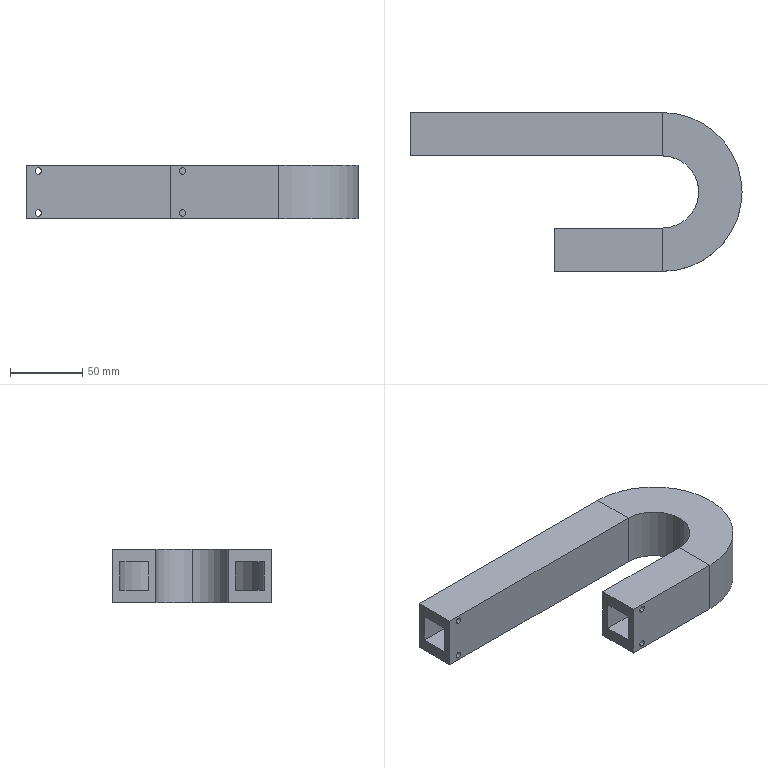Part | SolidWorks | features HoleWzd 2, Sweep 1 | 1 solid | 38 faces | box 230 x 110 x 37 mm | volume 264813 mm3 | plane 22 | cylinder 16 | commonest cylinder face diameters 4.5 x8 50 x2 60 x2 100 x2 110 x2
STEP:
#1=CARTESIAN_POINT('',(-91.5,65.,-12.25));
#2=VERTEX_POINT('',#1);
#3=CARTESIAN_POINT('',(-91.5,65.,-16.75));
#4=VERTEX_POINT('',#3);
#5=CARTESIAN_POINT('',(-91.5,65.,-14.5));
#6=DIRECTION('',(0.,-1.,0.));
#7=DIRECTION('',(1.,0.,0.));
#8=AXIS2_PLACEMENT_3D('',#5,#6,#7);
#9=CIRCLE('',#8,2.25);
#10=EDGE_CURVE('',#2,#4,#9,.T.);
#11=ORIENTED_EDGE('',*,*,#10,.T.);
#12=CARTESIAN_POINT('',(-91.5,95.,-16.75));
#13=VERTEX_POINT('',#12);
#14=CARTESIAN_POINT('',(-91.5,95.,-16.75));
#15=DIRECTION('',(0.,1.,0.));
#16=VECTOR('',#15,1000.);
#17=LINE('',#14,#16);
#18=EDGE_CURVE('',#4,#13,#17,.T.);
#19=ORIENTED_EDGE('',*,*,#18,.T.);
#20=CARTESIAN_POINT('',(-91.5,95.,-12.25));
#21=VERTEX_POINT('',#20);
#22=CARTESIAN_POINT('',(-91.5,95.,-14.5));
#23=DIRECTION('',(0.,1.,0.));
#24=DIRECTION('',(0.,0.,1.));
#25=AXIS2_PLACEMENT_3D('',#22,#23,#24);
#26=CIRCLE('',#25,2.25);
#27=EDGE_CURVE('',#13,#21,#26,.T.);
#28=ORIENTED_EDGE('',*,*,#27,.T.);
#29=CARTESIAN_POINT('',(-91.5,95.,-12.25));
#30=DIRECTION('',(0.,1.,0.));
#31=VECTOR('',#30,1000.);
#32=LINE('',#29,#31);
#33=EDGE_CURVE('',#2,#21,#32,.T.);
#34=ORIENTED_EDGE('',*,*,#33,.F.);
#35=EDGE_LOOP('',(#11,#19,#28,#34));
#36=FACE_OUTER_BOUND('',#35,.T.);
#37=CARTESIAN_POINT('',(-91.5,95.,-14.5));
#38=DIRECTION('',(0.,1.,0.));
#39=DIRECTION('',(0.,0.,1.));
#40=AXIS2_PLACEMENT_3D('',#37,#38,#39);
#41=CYLINDRICAL_SURFACE('',#40,2.25);
#42=ADVANCED_FACE('',(#36),#41,.F.);
#43=CARTESIAN_POINT('',(-91.5,65.,16.75));
#44=VERTEX_POINT('',#43);
#45=CARTESIAN_POINT('',(-91.5,65.,12.25));
#46=VERTEX_POINT('',#45);
#47=CARTESIAN_POINT('',(-91.5,65.,14.5));
#48=DIRECTION('',(0.,-1.,0.));
#49=DIRECTION('',(1.,0.,0.));
#50=AXIS2_PLACEMENT_3D('',#47,#48,#49);
#51=CIRCLE('',#50,2.25);
#52=EDGE_CURVE('',#44,#46,#51,.T.);
#53=ORIENTED_EDGE('',*,*,#52,.T.);
#54=CARTESIAN_POINT('',(-91.5,95.,12.25));
#55=VERTEX_POINT('',#54);
#56=CARTESIAN_POINT('',(-91.5,95.,12.25));
#57=DIRECTION('',(0.,1.,0.));
#58=VECTOR('',#57,1000.);
#59=LINE('',#56,#58);
#60=EDGE_CURVE('',#46,#55,#59,.T.);
#61=ORIENTED_EDGE('',*,*,#60,.T.);
#62=CARTESIAN_POINT('',(-91.5,95.,16.75));
#63=VERTEX_POINT('',#62);
#64=CARTESIAN_POINT('',(-91.5,95.,14.5));
#65=DIRECTION('',(0.,1.,0.));
#66=DIRECTION('',(0.,0.,1.));
#67=AXIS2_PLACEMENT_3D('',#64,#65,#66);
#68=CIRCLE('',#67,2.25);
#69=EDGE_CURVE('',#55,#63,#68,.T.);
#70=ORIENTED_EDGE('',*,*,#69,.T.);
#71=CARTESIAN_POINT('',(-91.5,95.,16.75));
#72=DIRECTION('',(0.,1.,0.));
#73=VECTOR('',#72,1000.);
#74=LINE('',#71,#73);
#75=EDGE_CURVE('',#44,#63,#74,.T.);
#76=ORIENTED_EDGE('',*,*,#75,.F.);
#77=EDGE_LOOP('',(#53,#61,#70,#76));
#78=FACE_OUTER_BOUND('',#77,.T.);
#79=CARTESIAN_POINT('',(-91.5,95.,14.5));
#80=DIRECTION('',(0.,1.,0.));
#81=DIRECTION('',(0.,0.,1.));
#82=AXIS2_PLACEMENT_3D('',#79,#80,#81);
#83=CYLINDRICAL_SURFACE('',#82,2.25);
#84=ADVANCED_FACE('',(#78),#83,.F.);
#85=CARTESIAN_POINT('',(8.5,-15.,-16.75));
#86=VERTEX_POINT('',#85);
#87=CARTESIAN_POINT('',(8.5,-15.,-12.25));
#88=VERTEX_POINT('',#87);
#89=CARTESIAN_POINT('',(8.5,-15.,-14.5));
#90=DIRECTION('',(0.,1.,0.));
#91=DIRECTION('',(0.,0.,1.));
#92=AXIS2_PLACEMENT_3D('',#89,#90,#91);
#93=CIRCLE('',#92,2.25);
#94=EDGE_CURVE('',#86,#88,#93,.T.);
#95=ORIENTED_EDGE('',*,*,#94,.F.);
#96=CARTESIAN_POINT('',(8.5,15.,-16.75));
#97=VERTEX_POINT('',#96);
#98=CARTESIAN_POINT('',(8.5,15.,-16.75));
#99=DIRECTION('',(0.,1.,0.));
#100=VECTOR('',#99,1000.);
#101=LINE('',#98,#100);
#102=EDGE_CURVE('',#86,#97,#101,.T.);
#103=ORIENTED_EDGE('',*,*,#102,.T.);
#104=CARTESIAN_POINT('',(8.5,15.,-12.25));
#105=VERTEX_POINT('',#104);
#106=CARTESIAN_POINT('',(8.5,15.,-14.5));
#107=DIRECTION('',(0.,1.,0.));
#108=DIRECTION('',(0.,0.,1.));
#109=AXIS2_PLACEMENT_3D('',#106,#107,#108);
#110=CIRCLE('',#109,2.25);
#111=EDGE_CURVE('',#97,#105,#110,.T.);
#112=ORIENTED_EDGE('',*,*,#111,.T.);
#113=CARTESIAN_POINT('',(8.5,15.,-12.25));
#114=DIRECTION('',(0.,1.,0.));
#115=VECTOR('',#114,1000.);
#116=LINE('',#113,#115);
#117=EDGE_CURVE('',#88,#105,#116,.T.);
#118=ORIENTED_EDGE('',*,*,#117,.F.);
#119=EDGE_LOOP('',(#95,#103,#112,#118));
#120=FACE_OUTER_BOUND('',#119,.T.);
#121=CARTESIAN_POINT('',(8.5,15.,-14.5));
#122=DIRECTION('',(0.,1.,0.));
#123=DIRECTION('',(0.,0.,1.));
#124=AXIS2_PLACEMENT_3D('',#121,#122,#123);
#125=CYLINDRICAL_SURFACE('',#124,2.25);
#126=ADVANCED_FACE('',(#120),#125,.F.);
#127=CARTESIAN_POINT('',(8.5,-15.,12.25));
#128=VERTEX_POINT('',#127);
#129=CARTESIAN_POINT('',(8.5,-15.,16.75));
#130=VERTEX_POINT('',#129);
#131=CARTESIAN_POINT('',(8.5,-15.,14.5));
#132=DIRECTION('',(0.,1.,0.));
#133=DIRECTION('',(0.,0.,1.));
#134=AXIS2_PLACEMENT_3D('',#131,#132,#133);
#135=CIRCLE('',#134,2.25);
#136=EDGE_CURVE('',#128,#130,#135,.T.);
#137=ORIENTED_EDGE('',*,*,#136,.F.);
#138=CARTESIAN_POINT('',(8.5,15.,12.25));
#139=VERTEX_POINT('',#138);
#140=CARTESIAN_POINT('',(8.5,15.,12.25));
#141=DIRECTION('',(0.,1.,0.));
#142=VECTOR('',#141,1000.);
#143=LINE('',#140,#142);
#144=EDGE_CURVE('',#128,#139,#143,.T.);
#145=ORIENTED_EDGE('',*,*,#144,.T.);
#146=CARTESIAN_POINT('',(8.5,15.,16.75));
#147=VERTEX_POINT('',#146);
#148=CARTESIAN_POINT('',(8.5,15.,14.5));
#149=DIRECTION('',(0.,1.,0.));
#150=DIRECTION('',(0.,0.,1.));
#151=AXIS2_PLACEMENT_3D('',#148,#149,#150);
#152=CIRCLE('',#151,2.25);
#153=EDGE_CURVE('',#139,#147,#152,.T.);
#154=ORIENTED_EDGE('',*,*,#153,.T.);
#155=CARTESIAN_POINT('',(8.5,15.,16.75));
#156=DIRECTION('',(0.,1.,0.));
#157=VECTOR('',#156,1000.);
#158=LINE('',#155,#157);
#159=EDGE_CURVE('',#130,#147,#158,.T.);
#160=ORIENTED_EDGE('',*,*,#159,.F.);
#161=EDGE_LOOP('',(#137,#145,#154,#160));
#162=FACE_OUTER_BOUND('',#161,.T.);
#163=CARTESIAN_POINT('',(8.5,15.,14.5));
#164=DIRECTION('',(0.,1.,0.));
#165=DIRECTION('',(0.,0.,1.));
#166=AXIS2_PLACEMENT_3D('',#163,#164,#165);
#167=CYLINDRICAL_SURFACE('',#166,2.25);
#168=ADVANCED_FACE('',(#162),#167,.F.);
#169=CARTESIAN_POINT('',(75.,10.,-10.));
#170=VERTEX_POINT('',#169);
#171=CARTESIAN_POINT('',(105.,40.,-10.));
#172=VERTEX_POINT('',#171);
#173=CARTESIAN_POINT('',(75.,40.,-10.));
#174=DIRECTION('',(0.,0.,1.));
#175=DIRECTION('',(0.,-1.,0.));
#176=AXIS2_PLACEMENT_3D('',#173,#174,#175);
#177=CIRCLE('',#176,30.);
#178=EDGE_CURVE('',#170,#172,#177,.T.);
#179=ORIENTED_EDGE('',*,*,#178,.T.);
#180=CARTESIAN_POINT('',(105.,40.,10.));
#181=VERTEX_POINT('',#180);
#182=CARTESIAN_POINT('',(105.,40.,0.));
#183=DIRECTION('',(0.,0.,1.));
#184=VECTOR('',#183,1000.);
#185=LINE('',#182,#184);
#186=EDGE_CURVE('',#172,#181,#185,.T.);
#187=ORIENTED_EDGE('',*,*,#186,.T.);
#188=CARTESIAN_POINT('',(75.,10.,10.));
#189=VERTEX_POINT('',#188);
#190=CARTESIAN_POINT('',(75.,40.,10.));
#191=DIRECTION('',(0.,0.,1.));
#192=DIRECTION('',(0.,-1.,0.));
#193=AXIS2_PLACEMENT_3D('',#190,#191,#192);
#194=CIRCLE('',#193,30.);
#195=EDGE_CURVE('',#189,#181,#194,.T.);
#196=ORIENTED_EDGE('',*,*,#195,.F.);
#197=CARTESIAN_POINT('',(75.,10.,10.));
#198=DIRECTION('',(0.,0.,-1.));
#199=VECTOR('',#198,1000.);
#200=LINE('',#197,#199);
#201=EDGE_CURVE('',#189,#170,#200,.T.);
#202=ORIENTED_EDGE('',*,*,#201,.T.);
#203=EDGE_LOOP('',(#179,#187,#196,#202));
#204=FACE_OUTER_BOUND('',#203,.T.);
#205=CARTESIAN_POINT('',(75.,40.,0.));
#206=DIRECTION('',(0.,0.,1.));
#207=DIRECTION('',(1.,0.,0.));
#208=AXIS2_PLACEMENT_3D('',#205,#206,#207);
#209=CYLINDRICAL_SURFACE('',#208,30.);
#210=ADVANCED_FACE('',(#204),#209,.T.);
#211=CARTESIAN_POINT('',(125.,40.,-10.));
#212=VERTEX_POINT('',#211);
#213=CARTESIAN_POINT('',(75.,90.,-10.));
#214=VERTEX_POINT('',#213);
#215=CARTESIAN_POINT('',(75.,40.,-10.));
#216=DIRECTION('',(0.,0.,1.));
#217=DIRECTION('',(0.,-1.,0.));
#218=AXIS2_PLACEMENT_3D('',#215,#216,#217);
#219=CIRCLE('',#218,50.);
#220=EDGE_CURVE('',#212,#214,#219,.T.);
#221=ORIENTED_EDGE('',*,*,#220,.F.);
#222=CARTESIAN_POINT('',(125.,40.,10.));
#223=VERTEX_POINT('',#222);
#224=CARTESIAN_POINT('',(125.,40.,0.));
#225=DIRECTION('',(0.,0.,1.));
#226=VECTOR('',#225,1000.);
#227=LINE('',#224,#226);
#228=EDGE_CURVE('',#212,#223,#227,.T.);
#229=ORIENTED_EDGE('',*,*,#228,.T.);
#230=CARTESIAN_POINT('',(75.,90.,10.));
#231=VERTEX_POINT('',#230);
#232=CARTESIAN_POINT('',(75.,40.,10.));
#233=DIRECTION('',(0.,0.,1.));
#234=DIRECTION('',(0.,-1.,0.));
#235=AXIS2_PLACEMENT_3D('',#232,#233,#234);
#236=CIRCLE('',#235,50.);
#237=EDGE_CURVE('',#223,#231,#236,.T.);
#238=ORIENTED_EDGE('',*,*,#237,.T.);
#239=CARTESIAN_POINT('',(75.,90.,10.));
#240=DIRECTION('',(0.,0.,1.));
#241=VECTOR('',#240,1000.);
#242=LINE('',#239,#241);
#243=EDGE_CURVE('',#214,#231,#242,.T.);
#244=ORIENTED_EDGE('',*,*,#243,.F.);
#245=EDGE_LOOP('',(#221,#229,#238,#244));
#246=FACE_OUTER_BOUND('',#245,.T.);
#247=CARTESIAN_POINT('',(75.,40.,0.));
#248=DIRECTION('',(0.,0.,1.));
#249=DIRECTION('',(1.,0.,0.));
#250=AXIS2_PLACEMENT_3D('',#247,#248,#249);
#251=CYLINDRICAL_SURFACE('',#250,50.);
#252=ADVANCED_FACE('',(#246),#251,.F.);
#253=CARTESIAN_POINT('',(75.,-15.,-18.5));
#254=VERTEX_POINT('',#253);
#255=CARTESIAN_POINT('',(130.,40.,-18.5));
#256=VERTEX_POINT('',#255);
#257=CARTESIAN_POINT('',(75.,40.,-18.5));
#258=DIRECTION('',(0.,0.,1.));
#259=DIRECTION('',(0.,-1.,0.));
#260=AXIS2_PLACEMENT_3D('',#257,#258,#259);
#261=CIRCLE('',#260,55.);
#262=EDGE_CURVE('',#254,#256,#261,.T.);
#263=ORIENTED_EDGE('',*,*,#262,.T.);
#264=CARTESIAN_POINT('',(130.,40.,18.5));
#265=VERTEX_POINT('',#264);
#266=CARTESIAN_POINT('',(130.,40.,0.));
#267=DIRECTION('',(0.,0.,1.));
#268=VECTOR('',#267,1000.);
#269=LINE('',#266,#268);
#270=EDGE_CURVE('',#256,#265,#269,.T.);
#271=ORIENTED_EDGE('',*,*,#270,.T.);
#272=CARTESIAN_POINT('',(75.,-15.,18.5));
#273=VERTEX_POINT('',#272);
#274=CARTESIAN_POINT('',(75.,40.,18.5));
#275=DIRECTION('',(0.,0.,1.));
#276=DIRECTION('',(0.,-1.,0.));
#277=AXIS2_PLACEMENT_3D('',#274,#275,#276);
#278=CIRCLE('',#277,55.);
#279=EDGE_CURVE('',#273,#265,#278,.T.);
#280=ORIENTED_EDGE('',*,*,#279,.F.);
#281=CARTESIAN_POINT('',(75.,-15.,18.5));
#282=DIRECTION('',(0.,0.,-1.));
#283=VECTOR('',#282,1000.);
#284=LINE('',#281,#283);
#285=EDGE_CURVE('',#273,#254,#284,.T.);
#286=ORIENTED_EDGE('',*,*,#285,.T.);
#287=EDGE_LOOP('',(#263,#271,#280,#286));
#288=FACE_OUTER_BOUND('',#287,.T.);
#289=CARTESIAN_POINT('',(75.,40.,0.));
#290=DIRECTION('',(0.,0.,1.));
#291=DIRECTION('',(1.,0.,0.));
#292=AXIS2_PLACEMENT_3D('',#289,#290,#291);
#293=CYLINDRICAL_SURFACE('',#292,55.);
#294=ADVANCED_FACE('',(#288),#293,.T.);
#295=CARTESIAN_POINT('',(100.,40.,-18.5));
#296=VERTEX_POINT('',#295);
#297=CARTESIAN_POINT('',(75.,65.,-18.5));
#298=VERTEX_POINT('',#297);
#299=CARTESIAN_POINT('',(75.,40.,-18.5));
#300=DIRECTION('',(0.,0.,1.));
#301=DIRECTION('',(0.,-1.,0.));
#302=AXIS2_PLACEMENT_3D('',#299,#300,#301);
#303=CIRCLE('',#302,25.);
#304=EDGE_CURVE('',#296,#298,#303,.T.);
#305=ORIENTED_EDGE('',*,*,#304,.F.);
#306=CARTESIAN_POINT('',(100.,40.,18.5));
#307=VERTEX_POINT('',#306);
#308=CARTESIAN_POINT('',(100.,40.,0.));
#309=DIRECTION('',(0.,0.,1.));
#310=VECTOR('',#309,1000.);
#311=LINE('',#308,#310);
#312=EDGE_CURVE('',#296,#307,#311,.T.);
#313=ORIENTED_EDGE('',*,*,#312,.T.);
#314=CARTESIAN_POINT('',(75.,65.,18.5));
#315=VERTEX_POINT('',#314);
#316=CARTESIAN_POINT('',(75.,40.,18.5));
#317=DIRECTION('',(0.,0.,1.));
#318=DIRECTION('',(0.,-1.,0.));
#319=AXIS2_PLACEMENT_3D('',#316,#317,#318);
#320=CIRCLE('',#319,25.);
#321=EDGE_CURVE('',#307,#315,#320,.T.);
#322=ORIENTED_EDGE('',*,*,#321,.T.);
#323=CARTESIAN_POINT('',(75.,65.,18.5));
#324=DIRECTION('',(0.,0.,1.));
#325=VECTOR('',#324,1000.);
#326=LINE('',#323,#325);
#327=EDGE_CURVE('',#298,#315,#326,.T.);
#328=ORIENTED_EDGE('',*,*,#327,.F.);
#329=EDGE_LOOP('',(#305,#313,#322,#328));
#330=FACE_OUTER_BOUND('',#329,.T.);
#331=CARTESIAN_POINT('',(75.,40.,0.));
#332=DIRECTION('',(0.,0.,1.));
#333=DIRECTION('',(1.,0.,0.));
#334=AXIS2_PLACEMENT_3D('',#331,#332,#333);
#335=CYLINDRICAL_SURFACE('',#334,25.);
#336=ADVANCED_FACE('',(#330),#335,.F.);
#337=CARTESIAN_POINT('',(-100.,70.,-10.));
#338=VERTEX_POINT('',#337);
#339=CARTESIAN_POINT('',(-100.,90.,-10.));
#340=VERTEX_POINT('',#339);
#341=CARTESIAN_POINT('',(-100.,90.,-10.));
#342=DIRECTION('',(0.,1.,0.));
#343=VECTOR('',#342,1000.);
#344=LINE('',#341,#343);
#345=EDGE_CURVE('',#338,#340,#344,.T.);
#346=ORIENTED_EDGE('',*,*,#345,.F.);
#347=CARTESIAN_POINT('',(75.,70.,-10.));
#348=VERTEX_POINT('',#347);
#349=CARTESIAN_POINT('',(75.,70.,-10.));
#350=DIRECTION('',(-1.,0.,0.));
#351=VECTOR('',#350,1000.);
#352=LINE('',#349,#351);
#353=EDGE_CURVE('',#348,#338,#352,.T.);
#354=ORIENTED_EDGE('',*,*,#353,.F.);
#355=CARTESIAN_POINT('',(75.,90.,-10.));
#356=DIRECTION('',(0.,1.,0.));
#357=VECTOR('',#356,1000.);
#358=LINE('',#355,#357);
#359=EDGE_CURVE('',#348,#214,#358,.T.);
#360=ORIENTED_EDGE('',*,*,#359,.T.);
#361=CARTESIAN_POINT('',(75.,90.,-10.));
#362=DIRECTION('',(-1.,0.,0.));
#363=VECTOR('',#362,1000.);
#364=LINE('',#361,#363);
#365=EDGE_CURVE('',#214,#340,#364,.T.);
#366=ORIENTED_EDGE('',*,*,#365,.T.);
#367=EDGE_LOOP('',(#346,#354,#360,#366));
#368=FACE_OUTER_BOUND('',#367,.T.);
#369=CARTESIAN_POINT('',(75.,90.,-10.));
#370=DIRECTION('',(0.,0.,1.));
#371=DIRECTION('',(1.,0.,0.));
#372=AXIS2_PLACEMENT_3D('',#369,#370,#371);
#373=PLANE('',#372);
#374=ADVANCED_FACE('',(#368),#373,.T.);
#375=ORIENTED_EDGE('',*,*,#353,.T.);
#376=CARTESIAN_POINT('',(-100.,70.,10.));
#377=VERTEX_POINT('',#376);
#378=CARTESIAN_POINT('',(-100.,70.,10.));
#379=DIRECTION('',(0.,0.,-1.));
#380=VECTOR('',#379,1000.);
#381=LINE('',#378,#380);
#382=EDGE_CURVE('',#377,#338,#381,.T.);
#383=ORIENTED_EDGE('',*,*,#382,.F.);
#384=CARTESIAN_POINT('',(75.,70.,10.));
#385=VERTEX_POINT('',#384);
#386=CARTESIAN_POINT('',(75.,70.,10.));
#387=DIRECTION('',(-1.,0.,0.));
#388=VECTOR('',#387,1000.);
#389=LINE('',#386,#388);
#390=EDGE_CURVE('',#385,#377,#389,.T.);
#391=ORIENTED_EDGE('',*,*,#390,.F.);
#392=CARTESIAN_POINT('',(75.,70.,10.));
#393=DIRECTION('',(0.,0.,-1.));
#394=VECTOR('',#393,1000.);
#395=LINE('',#392,#394);
#396=EDGE_CURVE('',#385,#348,#395,.T.);
#397=ORIENTED_EDGE('',*,*,#396,.T.);
#398=EDGE_LOOP('',(#375,#383,#391,#397));
#399=FACE_OUTER_BOUND('',#398,.T.);
#400=CARTESIAN_POINT('',(75.,70.,10.));
#401=DIRECTION('',(0.,1.,0.));
#402=DIRECTION('',(-1.,0.,0.));
#403=AXIS2_PLACEMENT_3D('',#400,#401,#402);
#404=PLANE('',#403);
#405=ADVANCED_FACE('',(#399),#404,.T.);
#406=ORIENTED_EDGE('',*,*,#390,.T.);
#407=CARTESIAN_POINT('',(-100.,90.,10.));
#408=VERTEX_POINT('',#407);
#409=CARTESIAN_POINT('',(-100.,90.,10.));
#410=DIRECTION('',(0.,-1.,0.));
#411=VECTOR('',#410,1000.);
#412=LINE('',#409,#411);
#413=EDGE_CURVE('',#408,#377,#412,.T.);
#414=ORIENTED_EDGE('',*,*,#413,.F.);
#415=CARTESIAN_POINT('',(75.,90.,10.));
#416=DIRECTION('',(-1.,0.,0.));
#417=VECTOR('',#416,1000.);
#418=LINE('',#415,#417);
#419=EDGE_CURVE('',#231,#408,#418,.T.);
#420=ORIENTED_EDGE('',*,*,#419,.F.);
#421=CARTESIAN_POINT('',(75.,90.,10.));
#422=DIRECTION('',(0.,-1.,0.));
#423=VECTOR('',#422,1000.);
#424=LINE('',#421,#423);
#425=EDGE_CURVE('',#231,#385,#424,.T.);
#426=ORIENTED_EDGE('',*,*,#425,.T.);
#427=EDGE_LOOP('',(#406,#414,#420,#426));
#428=FACE_OUTER_BOUND('',#427,.T.);
#429=CARTESIAN_POINT('',(75.,90.,10.));
#430=DIRECTION('',(0.,0.,-1.));
#431=DIRECTION('',(-1.,0.,0.));
#432=AXIS2_PLACEMENT_3D('',#429,#430,#431);
#433=PLANE('',#432);
#434=ADVANCED_FACE('',(#428),#433,.T.);
#435=ORIENTED_EDGE('',*,*,#419,.T.);
#436=CARTESIAN_POINT('',(-100.,90.,10.));
#437=DIRECTION('',(0.,0.,1.));
#438=VECTOR('',#437,1000.);
#439=LINE('',#436,#438);
#440=EDGE_CURVE('',#340,#408,#439,.T.);
#441=ORIENTED_EDGE('',*,*,#440,.F.);
#442=ORIENTED_EDGE('',*,*,#365,.F.);
#443=ORIENTED_EDGE('',*,*,#243,.T.);
#444=EDGE_LOOP('',(#435,#441,#442,#443));
#445=FACE_OUTER_BOUND('',#444,.T.);
#446=CARTESIAN_POINT('',(75.,90.,10.));
#447=DIRECTION('',(0.,-1.,0.));
#448=DIRECTION('',(1.,0.,0.));
#449=AXIS2_PLACEMENT_3D('',#446,#447,#448);
#450=PLANE('',#449);
#451=ADVANCED_FACE('',(#445),#450,.T.);
#452=ORIENTED_EDGE('',*,*,#359,.F.);
#453=CARTESIAN_POINT('',(75.,40.,-10.));
#454=DIRECTION('',(0.,0.,1.));
#455=DIRECTION('',(0.,-1.,0.));
#456=AXIS2_PLACEMENT_3D('',#453,#454,#455);
#457=CIRCLE('',#456,30.);
#458=EDGE_CURVE('',#172,#348,#457,.T.);
#459=ORIENTED_EDGE('',*,*,#458,.F.);
#460=ORIENTED_EDGE('',*,*,#178,.F.);
#461=CARTESIAN_POINT('',(75.,-10.,-10.));
#462=VERTEX_POINT('',#461);
#463=CARTESIAN_POINT('',(75.,-10.,-10.));
#464=DIRECTION('',(0.,-1.,0.));
#465=VECTOR('',#464,1000.);
#466=LINE('',#463,#465);
#467=EDGE_CURVE('',#170,#462,#466,.T.);
#468=ORIENTED_EDGE('',*,*,#467,.T.);
#469=CARTESIAN_POINT('',(75.,40.,-10.));
#470=DIRECTION('',(0.,0.,1.));
#471=DIRECTION('',(0.,-1.,0.));
#472=AXIS2_PLACEMENT_3D('',#469,#470,#471);
#473=CIRCLE('',#472,50.);
#474=EDGE_CURVE('',#462,#212,#473,.T.);
#475=ORIENTED_EDGE('',*,*,#474,.T.);
#476=ORIENTED_EDGE('',*,*,#220,.T.);
#477=EDGE_LOOP('',(#452,#459,#460,#468,#475,#476));
#478=FACE_OUTER_BOUND('',#477,.T.);
#479=CARTESIAN_POINT('',(75.,-10.,-10.));
#480=DIRECTION('',(0.,0.,1.));
#481=DIRECTION('',(1.,0.,0.));
#482=AXIS2_PLACEMENT_3D('',#479,#480,#481);
#483=PLANE('',#482);
#484=ADVANCED_FACE('',(#478),#483,.T.);
#485=ORIENTED_EDGE('',*,*,#186,.F.);
#486=ORIENTED_EDGE('',*,*,#458,.T.);
#487=ORIENTED_EDGE('',*,*,#396,.F.);
#488=CARTESIAN_POINT('',(75.,40.,10.));
#489=DIRECTION('',(0.,0.,1.));
#490=DIRECTION('',(0.,-1.,0.));
#491=AXIS2_PLACEMENT_3D('',#488,#489,#490);
#492=CIRCLE('',#491,30.);
#493=EDGE_CURVE('',#181,#385,#492,.T.);
#494=ORIENTED_EDGE('',*,*,#493,.F.);
#495=EDGE_LOOP('',(#485,#486,#487,#494));
#496=FACE_OUTER_BOUND('',#495,.T.);
#497=CARTESIAN_POINT('',(75.,40.,0.));
#498=DIRECTION('',(0.,0.,1.));
#499=DIRECTION('',(1.,0.,0.));
#500=AXIS2_PLACEMENT_3D('',#497,#498,#499);
#501=CYLINDRICAL_SURFACE('',#500,30.);
#502=ADVANCED_FACE('',(#496),#501,.T.);
#503=ORIENTED_EDGE('',*,*,#195,.T.);
#504=ORIENTED_EDGE('',*,*,#493,.T.);
#505=ORIENTED_EDGE('',*,*,#425,.F.);
#506=ORIENTED_EDGE('',*,*,#237,.F.);
#507=CARTESIAN_POINT('',(75.,-10.,10.));
#508=VERTEX_POINT('',#507);
#509=CARTESIAN_POINT('',(75.,40.,10.));
#510=DIRECTION('',(0.,0.,1.));
#511=DIRECTION('',(0.,-1.,0.));
#512=AXIS2_PLACEMENT_3D('',#509,#510,#511);
#513=CIRCLE('',#512,50.);
#514=EDGE_CURVE('',#508,#223,#513,.T.);
#515=ORIENTED_EDGE('',*,*,#514,.F.);
#516=CARTESIAN_POINT('',(75.,-10.,10.));
#517=DIRECTION('',(0.,1.,0.));
#518=VECTOR('',#517,1000.);
#519=LINE('',#516,#518);
#520=EDGE_CURVE('',#508,#189,#519,.T.);
#521=ORIENTED_EDGE('',*,*,#520,.T.);
#522=EDGE_LOOP('',(#503,#504,#505,#506,#515,#521));
#523=FACE_OUTER_BOUND('',#522,.T.);
#524=CARTESIAN_POINT('',(75.,-10.,10.));
#525=DIRECTION('',(0.,0.,-1.));
#526=DIRECTION('',(-1.,0.,0.));
#527=AXIS2_PLACEMENT_3D('',#524,#525,#526);
#528=PLANE('',#527);
#529=ADVANCED_FACE('',(#523),#528,.T.);
#530=ORIENTED_EDGE('',*,*,#228,.F.);
#531=ORIENTED_EDGE('',*,*,#474,.F.);
#532=CARTESIAN_POINT('',(75.,-10.,10.));
#533=DIRECTION('',(0.,0.,1.));
#534=VECTOR('',#533,1000.);
#535=LINE('',#532,#534);
#536=EDGE_CURVE('',#462,#508,#535,.T.);
#537=ORIENTED_EDGE('',*,*,#536,.T.);
#538=ORIENTED_EDGE('',*,*,#514,.T.);
#539=EDGE_LOOP('',(#530,#531,#537,#538));
#540=FACE_OUTER_BOUND('',#539,.T.);
#541=CARTESIAN_POINT('',(75.,40.,0.));
#542=DIRECTION('',(0.,0.,1.));
#543=DIRECTION('',(1.,0.,0.));
#544=AXIS2_PLACEMENT_3D('',#541,#542,#543);
#545=CYLINDRICAL_SURFACE('',#544,50.);
#546=ADVANCED_FACE('',(#540),#545,.F.);
#547=ORIENTED_EDGE('',*,*,#467,.F.);
#548=CARTESIAN_POINT('',(0.,10.,-10.));
#549=VERTEX_POINT('',#548);
#550=CARTESIAN_POINT('',(0.,10.,-10.));
#551=DIRECTION('',(1.,0.,0.));
#552=VECTOR('',#551,1000.);
#553=LINE('',#550,#552);
#554=EDGE_CURVE('',#549,#170,#553,.T.);
#555=ORIENTED_EDGE('',*,*,#554,.F.);
#556=CARTESIAN_POINT('',(0.,-10.,-10.));
#557=VERTEX_POINT('',#556);
#558=CARTESIAN_POINT('',(0.,-10.,-10.));
#559=DIRECTION('',(0.,-1.,0.));
#560=VECTOR('',#559,1000.);
#561=LINE('',#558,#560);
#562=EDGE_CURVE('',#549,#557,#561,.T.);
#563=ORIENTED_EDGE('',*,*,#562,.T.);
#564=CARTESIAN_POINT('',(0.,-10.,-10.));
#565=DIRECTION('',(1.,0.,0.));
#566=VECTOR('',#565,1000.);
#567=LINE('',#564,#566);
#568=EDGE_CURVE('',#557,#462,#567,.T.);
#569=ORIENTED_EDGE('',*,*,#568,.T.);
#570=EDGE_LOOP('',(#547,#555,#563,#569));
#571=FACE_OUTER_BOUND('',#570,.T.);
#572=CARTESIAN_POINT('',(0.,-10.,-10.));
#573=DIRECTION('',(0.,0.,1.));
#574=DIRECTION('',(1.,0.,0.));
#575=AXIS2_PLACEMENT_3D('',#572,#573,#574);
#576=PLANE('',#575);
#577=ADVANCED_FACE('',(#571),#576,.T.);
#578=ORIENTED_EDGE('',*,*,#554,.T.);
#579=ORIENTED_EDGE('',*,*,#201,.F.);
#580=CARTESIAN_POINT('',(0.,10.,10.));
#581=VERTEX_POINT('',#580);
#582=CARTESIAN_POINT('',(0.,10.,10.));
#583=DIRECTION('',(1.,0.,0.));
#584=VECTOR('',#583,1000.);
#585=LINE('',#582,#584);
#586=EDGE_CURVE('',#581,#189,#585,.T.);
#587=ORIENTED_EDGE('',*,*,#586,.F.);
#588=CARTESIAN_POINT('',(0.,10.,10.));
#589=DIRECTION('',(0.,0.,-1.));
#590=VECTOR('',#589,1000.);
#591=LINE('',#588,#590);
#592=EDGE_CURVE('',#581,#549,#591,.T.);
#593=ORIENTED_EDGE('',*,*,#592,.T.);
#594=EDGE_LOOP('',(#578,#579,#587,#593));
#595=FACE_OUTER_BOUND('',#594,.T.);
#596=CARTESIAN_POINT('',(0.,10.,10.));
#597=DIRECTION('',(0.,-1.,0.));
#598=DIRECTION('',(0.,0.,-1.));
#599=AXIS2_PLACEMENT_3D('',#596,#597,#598);
#600=PLANE('',#599);
#601=ADVANCED_FACE('',(#595),#600,.T.);
#602=ORIENTED_EDGE('',*,*,#586,.T.);
#603=ORIENTED_EDGE('',*,*,#520,.F.);
#604=CARTESIAN_POINT('',(0.,-10.,10.));
#605=VERTEX_POINT('',#604);
#606=CARTESIAN_POINT('',(0.,-10.,10.));
#607=DIRECTION('',(1.,0.,0.));
#608=VECTOR('',#607,1000.);
#609=LINE('',#606,#608);
#610=EDGE_CURVE('',#605,#508,#609,.T.);
#611=ORIENTED_EDGE('',*,*,#610,.F.);
#612=CARTESIAN_POINT('',(0.,-10.,10.));
#613=DIRECTION('',(0.,1.,0.));
#614=VECTOR('',#613,1000.);
#615=LINE('',#612,#614);
#616=EDGE_CURVE('',#605,#581,#615,.T.);
#617=ORIENTED_EDGE('',*,*,#616,.T.);
#618=EDGE_LOOP('',(#602,#603,#611,#617));
#619=FACE_OUTER_BOUND('',#618,.T.);
#620=CARTESIAN_POINT('',(0.,-10.,10.));
#621=DIRECTION('',(0.,0.,-1.));
#622=DIRECTION('',(-1.,0.,0.));
#623=AXIS2_PLACEMENT_3D('',#620,#621,#622);
#624=PLANE('',#623);
#625=ADVANCED_FACE('',(#619),#624,.T.);
#626=ORIENTED_EDGE('',*,*,#610,.T.);
#627=ORIENTED_EDGE('',*,*,#536,.F.);
#628=ORIENTED_EDGE('',*,*,#568,.F.);
#629=CARTESIAN_POINT('',(0.,-10.,10.));
#630=DIRECTION('',(0.,0.,1.));
#631=VECTOR('',#630,1000.);
#632=LINE('',#629,#631);
#633=EDGE_CURVE('',#557,#605,#632,.T.);
#634=ORIENTED_EDGE('',*,*,#633,.T.);
#635=EDGE_LOOP('',(#626,#627,#628,#634));
#636=FACE_OUTER_BOUND('',#635,.T.);
#637=CARTESIAN_POINT('',(0.,-10.,10.));
#638=DIRECTION('',(0.,1.,0.));
#639=DIRECTION('',(0.,0.,1.));
#640=AXIS2_PLACEMENT_3D('',#637,#638,#639);
#641=PLANE('',#640);
#642=ADVANCED_FACE('',(#636),#641,.T.);
#643=CARTESIAN_POINT('',(-100.,95.,-18.5));
#644=VERTEX_POINT('',#643);
#645=CARTESIAN_POINT('',(-100.,65.,-18.5));
#646=VERTEX_POINT('',#645);
#647=CARTESIAN_POINT('',(-100.,95.,-18.5));
#648=DIRECTION('',(0.,-1.,0.));
#649=VECTOR('',#648,1000.);
#650=LINE('',#647,#649);
#651=EDGE_CURVE('',#644,#646,#650,.T.);
#652=ORIENTED_EDGE('',*,*,#651,.T.);
#653=CARTESIAN_POINT('',(-100.,65.,18.5));
#654=VERTEX_POINT('',#653);
#655=CARTESIAN_POINT('',(-100.,65.,18.5));
#656=DIRECTION('',(0.,0.,1.));
#657=VECTOR('',#656,1000.);
#658=LINE('',#655,#657);
#659=EDGE_CURVE('',#646,#654,#658,.T.);
#660=ORIENTED_EDGE('',*,*,#659,.T.);
#661=CARTESIAN_POINT('',(-100.,95.,18.5));
#662=VERTEX_POINT('',#661);
#663=CARTESIAN_POINT('',(-100.,95.,18.5));
#664=DIRECTION('',(0.,1.,0.));
#665=VECTOR('',#664,1000.);
#666=LINE('',#663,#665);
#667=EDGE_CURVE('',#654,#662,#666,.T.);
#668=ORIENTED_EDGE('',*,*,#667,.T.);
#669=CARTESIAN_POINT('',(-100.,95.,18.5));
#670=DIRECTION('',(0.,0.,-1.));
#671=VECTOR('',#670,1000.);
#672=LINE('',#669,#671);
#673=EDGE_CURVE('',#662,#644,#672,.T.);
#674=ORIENTED_EDGE('',*,*,#673,.T.);
#675=EDGE_LOOP('',(#652,#660,#668,#674));
#676=FACE_OUTER_BOUND('',#675,.T.);
#677=ORIENTED_EDGE('',*,*,#345,.T.);
#678=ORIENTED_EDGE('',*,*,#440,.T.);
#679=ORIENTED_EDGE('',*,*,#413,.T.);
#680=ORIENTED_EDGE('',*,*,#382,.T.);
#681=EDGE_LOOP('',(#677,#678,#679,#680));
#682=FACE_BOUND('',#681,.T.);
#683=CARTESIAN_POINT('',(-100.,80.,0.));
#684=DIRECTION('',(1.,0.,0.));
#685=DIRECTION('',(0.,0.,1.));
#686=AXIS2_PLACEMENT_3D('',#683,#684,#685);
#687=PLANE('',#686);
#688=ADVANCED_FACE('',(#676,#682),#687,.F.);
#689=CARTESIAN_POINT('',(0.,-15.,-18.5));
#690=VERTEX_POINT('',#689);
#691=CARTESIAN_POINT('',(0.,15.,-18.5));
#692=VERTEX_POINT('',#691);
#693=CARTESIAN_POINT('',(0.,-15.,-18.5));
#694=DIRECTION('',(0.,1.,0.));
#695=VECTOR('',#694,1000.);
#696=LINE('',#693,#695);
#697=EDGE_CURVE('',#690,#692,#696,.T.);
#698=ORIENTED_EDGE('',*,*,#697,.F.);
#699=CARTESIAN_POINT('',(0.,-15.,18.5));
#700=VERTEX_POINT('',#699);
#701=CARTESIAN_POINT('',(0.,-15.,18.5));
#702=DIRECTION('',(0.,0.,-1.));
#703=VECTOR('',#702,1000.);
#704=LINE('',#701,#703);
#705=EDGE_CURVE('',#700,#690,#704,.T.);
#706=ORIENTED_EDGE('',*,*,#705,.F.);
#707=CARTESIAN_POINT('',(0.,15.,18.5));
#708=VERTEX_POINT('',#707);
#709=CARTESIAN_POINT('',(0.,-15.,18.5));
#710=DIRECTION('',(0.,-1.,0.));
#711=VECTOR('',#710,1000.);
#712=LINE('',#709,#711);
#713=EDGE_CURVE('',#708,#700,#712,.T.);
#714=ORIENTED_EDGE('',*,*,#713,.F.);
#715=CARTESIAN_POINT('',(0.,15.,18.5));
#716=DIRECTION('',(0.,0.,1.));
#717=VECTOR('',#716,1000.);
#718=LINE('',#715,#717);
#719=EDGE_CURVE('',#692,#708,#718,.T.);
#720=ORIENTED_EDGE('',*,*,#719,.F.);
#721=EDGE_LOOP('',(#698,#706,#714,#720));
#722=FACE_OUTER_BOUND('',#721,.T.);
#723=ORIENTED_EDGE('',*,*,#562,.F.);
#724=ORIENTED_EDGE('',*,*,#592,.F.);
#725=ORIENTED_EDGE('',*,*,#616,.F.);
#726=ORIENTED_EDGE('',*,*,#633,.F.);
#727=EDGE_LOOP('',(#723,#724,#725,#726));
#728=FACE_BOUND('',#727,.T.);
#729=CARTESIAN_POINT('',(0.,0.,0.));
#730=DIRECTION('',(-1.,0.,0.));
#731=DIRECTION('',(0.,0.,1.));
#732=AXIS2_PLACEMENT_3D('',#729,#730,#731);
#733=PLANE('',#732);
#734=ADVANCED_FACE('',(#722,#728),#733,.T.);
#735=CARTESIAN_POINT('',(-91.5,95.,-14.5));
#736=DIRECTION('',(0.,1.,0.));
#737=DIRECTION('',(0.,0.,1.));
#738=AXIS2_PLACEMENT_3D('',#735,#736,#737);
#739=CIRCLE('',#738,2.25);
#740=EDGE_CURVE('',#21,#13,#739,.T.);
#741=ORIENTED_EDGE('',*,*,#740,.F.);
#742=ORIENTED_EDGE('',*,*,#27,.F.);
#743=EDGE_LOOP('',(#741,#742));
#744=FACE_BOUND('',#743,.T.);
#745=CARTESIAN_POINT('',(-91.5,95.,14.5));
#746=DIRECTION('',(0.,1.,0.));
#747=DIRECTION('',(0.,0.,1.));
#748=AXIS2_PLACEMENT_3D('',#745,#746,#747);
#749=CIRCLE('',#748,2.25);
#750=EDGE_CURVE('',#63,#55,#749,.T.);
#751=ORIENTED_EDGE('',*,*,#750,.F.);
#752=ORIENTED_EDGE('',*,*,#69,.F.);
#753=EDGE_LOOP('',(#751,#752));
#754=FACE_BOUND('',#753,.T.);
#755=ORIENTED_EDGE('',*,*,#673,.F.);
#756=CARTESIAN_POINT('',(75.,95.,18.5));
#757=VERTEX_POINT('',#756);
#758=CARTESIAN_POINT('',(75.,95.,18.5));
#759=DIRECTION('',(-1.,0.,0.));
#760=VECTOR('',#759,1000.);
#761=LINE('',#758,#760);
#762=EDGE_CURVE('',#757,#662,#761,.T.);
#763=ORIENTED_EDGE('',*,*,#762,.F.);
#764=CARTESIAN_POINT('',(75.,95.,-18.5));
#765=VERTEX_POINT('',#764);
#766=CARTESIAN_POINT('',(75.,95.,18.5));
#767=DIRECTION('',(0.,0.,-1.));
#768=VECTOR('',#767,1000.);
#769=LINE('',#766,#768);
#770=EDGE_CURVE('',#757,#765,#769,.T.);
#771=ORIENTED_EDGE('',*,*,#770,.T.);
#772=CARTESIAN_POINT('',(75.,95.,-18.5));
#773=DIRECTION('',(-1.,0.,0.));
#774=VECTOR('',#773,1000.);
#775=LINE('',#772,#774);
#776=EDGE_CURVE('',#765,#644,#775,.T.);
#777=ORIENTED_EDGE('',*,*,#776,.T.);
#778=EDGE_LOOP('',(#755,#763,#771,#777));
#779=FACE_OUTER_BOUND('',#778,.T.);
#780=CARTESIAN_POINT('',(75.,95.,18.5));
#781=DIRECTION('',(0.,1.,0.));
#782=DIRECTION('',(-1.,0.,0.));
#783=AXIS2_PLACEMENT_3D('',#780,#781,#782);
#784=PLANE('',#783);
#785=ADVANCED_FACE('',(#744,#754,#779),#784,.T.);
#786=ORIENTED_EDGE('',*,*,#762,.T.);
#787=ORIENTED_EDGE('',*,*,#667,.F.);
#788=CARTESIAN_POINT('',(75.,65.,18.5));
#789=DIRECTION('',(-1.,0.,0.));
#790=VECTOR('',#789,1000.);
#791=LINE('',#788,#790);
#792=EDGE_CURVE('',#315,#654,#791,.T.);
#793=ORIENTED_EDGE('',*,*,#792,.F.);
#794=CARTESIAN_POINT('',(75.,95.,18.5));
#795=DIRECTION('',(0.,1.,0.));
#796=VECTOR('',#795,1000.);
#797=LINE('',#794,#796);
#798=EDGE_CURVE('',#315,#757,#797,.T.);
#799=ORIENTED_EDGE('',*,*,#798,.T.);
#800=EDGE_LOOP('',(#786,#787,#793,#799));
#801=FACE_OUTER_BOUND('',#800,.T.);
#802=CARTESIAN_POINT('',(75.,95.,18.5));
#803=DIRECTION('',(0.,0.,1.));
#804=DIRECTION('',(1.,0.,0.));
#805=AXIS2_PLACEMENT_3D('',#802,#803,#804);
#806=PLANE('',#805);
#807=ADVANCED_FACE('',(#801),#806,.T.);
#808=ORIENTED_EDGE('',*,*,#10,.F.);
#809=CARTESIAN_POINT('',(-91.5,65.,-14.5));
#810=DIRECTION('',(0.,-1.,0.));
#811=DIRECTION('',(1.,0.,0.));
#812=AXIS2_PLACEMENT_3D('',#809,#810,#811);
#813=CIRCLE('',#812,2.25);
#814=EDGE_CURVE('',#4,#2,#813,.T.);
#815=ORIENTED_EDGE('',*,*,#814,.F.);
#816=EDGE_LOOP('',(#808,#815));
#817=FACE_BOUND('',#816,.T.);
#818=ORIENTED_EDGE('',*,*,#52,.F.);
#819=CARTESIAN_POINT('',(-91.5,65.,14.5));
#820=DIRECTION('',(0.,-1.,0.));
#821=DIRECTION('',(1.,0.,0.));
#822=AXIS2_PLACEMENT_3D('',#819,#820,#821);
#823=CIRCLE('',#822,2.25);
#824=EDGE_CURVE('',#46,#44,#823,.T.);
#825=ORIENTED_EDGE('',*,*,#824,.F.);
#826=EDGE_LOOP('',(#818,#825));
#827=FACE_BOUND('',#826,.T.);
#828=ORIENTED_EDGE('',*,*,#792,.T.);
#829=ORIENTED_EDGE('',*,*,#659,.F.);
#830=CARTESIAN_POINT('',(75.,65.,-18.5));
#831=DIRECTION('',(-1.,0.,0.));
#832=VECTOR('',#831,1000.);
#833=LINE('',#830,#832);
#834=EDGE_CURVE('',#298,#646,#833,.T.);
#835=ORIENTED_EDGE('',*,*,#834,.F.);
#836=ORIENTED_EDGE('',*,*,#327,.T.);
#837=EDGE_LOOP('',(#828,#829,#835,#836));
#838=FACE_OUTER_BOUND('',#837,.T.);
#839=CARTESIAN_POINT('',(75.,65.,18.5));
#840=DIRECTION('',(0.,-1.,0.));
#841=DIRECTION('',(1.,0.,0.));
#842=AXIS2_PLACEMENT_3D('',#839,#840,#841);
#843=PLANE('',#842);
#844=ADVANCED_FACE('',(#817,#827,#838),#843,.T.);
#845=ORIENTED_EDGE('',*,*,#834,.T.);
#846=ORIENTED_EDGE('',*,*,#651,.F.);
#847=ORIENTED_EDGE('',*,*,#776,.F.);
#848=CARTESIAN_POINT('',(75.,95.,-18.5));
#849=DIRECTION('',(0.,-1.,0.));
#850=VECTOR('',#849,1000.);
#851=LINE('',#848,#850);
#852=EDGE_CURVE('',#765,#298,#851,.T.);
#853=ORIENTED_EDGE('',*,*,#852,.T.);
#854=EDGE_LOOP('',(#845,#846,#847,#853));
#855=FACE_OUTER_BOUND('',#854,.T.);
#856=CARTESIAN_POINT('',(75.,95.,-18.5));
#857=DIRECTION('',(0.,0.,-1.));
#858=DIRECTION('',(-1.,0.,0.));
#859=AXIS2_PLACEMENT_3D('',#856,#857,#858);
#860=PLANE('',#859);
#861=ADVANCED_FACE('',(#855),#860,.T.);
#862=ORIENTED_EDGE('',*,*,#270,.F.);
#863=CARTESIAN_POINT('',(75.,40.,-18.5));
#864=DIRECTION('',(0.,0.,1.));
#865=DIRECTION('',(0.,-1.,0.));
#866=AXIS2_PLACEMENT_3D('',#863,#864,#865);
#867=CIRCLE('',#866,55.);
#868=EDGE_CURVE('',#256,#765,#867,.T.);
#869=ORIENTED_EDGE('',*,*,#868,.T.);
#870=ORIENTED_EDGE('',*,*,#770,.F.);
#871=CARTESIAN_POINT('',(75.,40.,18.5));
#872=DIRECTION('',(0.,0.,1.));
#873=DIRECTION('',(0.,-1.,0.));
#874=AXIS2_PLACEMENT_3D('',#871,#872,#873);
#875=CIRCLE('',#874,55.);
#876=EDGE_CURVE('',#265,#757,#875,.T.);
#877=ORIENTED_EDGE('',*,*,#876,.F.);
#878=EDGE_LOOP('',(#862,#869,#870,#877));
#879=FACE_OUTER_BOUND('',#878,.T.);
#880=CARTESIAN_POINT('',(75.,40.,0.));
#881=DIRECTION('',(0.,0.,1.));
#882=DIRECTION('',(1.,0.,0.));
#883=AXIS2_PLACEMENT_3D('',#880,#881,#882);
#884=CYLINDRICAL_SURFACE('',#883,55.);
#885=ADVANCED_FACE('',(#879),#884,.T.);
#886=ORIENTED_EDGE('',*,*,#279,.T.);
#887=ORIENTED_EDGE('',*,*,#876,.T.);
#888=ORIENTED_EDGE('',*,*,#798,.F.);
#889=ORIENTED_EDGE('',*,*,#321,.F.);
#890=CARTESIAN_POINT('',(75.,15.,18.5));
#891=VERTEX_POINT('',#890);
#892=CARTESIAN_POINT('',(75.,40.,18.5));
#893=DIRECTION('',(0.,0.,1.));
#894=DIRECTION('',(0.,-1.,0.));
#895=AXIS2_PLACEMENT_3D('',#892,#893,#894);
#896=CIRCLE('',#895,25.);
#897=EDGE_CURVE('',#891,#307,#896,.T.);
#898=ORIENTED_EDGE('',*,*,#897,.F.);
#899=CARTESIAN_POINT('',(75.,-15.,18.5));
#900=DIRECTION('',(0.,-1.,0.));
#901=VECTOR('',#900,1000.);
#902=LINE('',#899,#901);
#903=EDGE_CURVE('',#891,#273,#902,.T.);
#904=ORIENTED_EDGE('',*,*,#903,.T.);
#905=EDGE_LOOP('',(#886,#887,#888,#889,#898,#904));
#906=FACE_OUTER_BOUND('',#905,.T.);
#907=CARTESIAN_POINT('',(75.,-15.,18.5));
#908=DIRECTION('',(0.,0.,1.));
#909=DIRECTION('',(1.,0.,0.));
#910=AXIS2_PLACEMENT_3D('',#907,#908,#909);
#911=PLANE('',#910);
#912=ADVANCED_FACE('',(#906),#911,.T.);
#913=ORIENTED_EDGE('',*,*,#312,.F.);
#914=CARTESIAN_POINT('',(75.,15.,-18.5));
#915=VERTEX_POINT('',#914);
#916=CARTESIAN_POINT('',(75.,40.,-18.5));
#917=DIRECTION('',(0.,0.,1.));
#918=DIRECTION('',(0.,-1.,0.));
#919=AXIS2_PLACEMENT_3D('',#916,#917,#918);
#920=CIRCLE('',#919,25.);
#921=EDGE_CURVE('',#915,#296,#920,.T.);
#922=ORIENTED_EDGE('',*,*,#921,.F.);
#923=CARTESIAN_POINT('',(75.,15.,18.5));
#924=DIRECTION('',(0.,0.,1.));
#925=VECTOR('',#924,1000.);
#926=LINE('',#923,#925);
#927=EDGE_CURVE('',#915,#891,#926,.T.);
#928=ORIENTED_EDGE('',*,*,#927,.T.);
#929=ORIENTED_EDGE('',*,*,#897,.T.);
#930=EDGE_LOOP('',(#913,#922,#928,#929));
#931=FACE_OUTER_BOUND('',#930,.T.);
#932=CARTESIAN_POINT('',(75.,40.,0.));
#933=DIRECTION('',(0.,0.,1.));
#934=DIRECTION('',(1.,0.,0.));
#935=AXIS2_PLACEMENT_3D('',#932,#933,#934);
#936=CYLINDRICAL_SURFACE('',#935,25.);
#937=ADVANCED_FACE('',(#931),#936,.F.);
#938=ORIENTED_EDGE('',*,*,#921,.T.);
#939=ORIENTED_EDGE('',*,*,#304,.T.);
#940=ORIENTED_EDGE('',*,*,#852,.F.);
#941=ORIENTED_EDGE('',*,*,#868,.F.);
#942=ORIENTED_EDGE('',*,*,#262,.F.);
#943=CARTESIAN_POINT('',(75.,-15.,-18.5));
#944=DIRECTION('',(0.,1.,0.));
#945=VECTOR('',#944,1000.);
#946=LINE('',#943,#945);
#947=EDGE_CURVE('',#254,#915,#946,.T.);
#948=ORIENTED_EDGE('',*,*,#947,.T.);
#949=EDGE_LOOP('',(#938,#939,#940,#941,#942,#948));
#950=FACE_OUTER_BOUND('',#949,.T.);
#951=CARTESIAN_POINT('',(75.,-15.,-18.5));
#952=DIRECTION('',(0.,0.,-1.));
#953=DIRECTION('',(-1.,0.,0.));
#954=AXIS2_PLACEMENT_3D('',#951,#952,#953);
#955=PLANE('',#954);
#956=ADVANCED_FACE('',(#950),#955,.T.);
#957=CARTESIAN_POINT('',(8.5,-15.,-14.5));
#958=DIRECTION('',(0.,1.,0.));
#959=DIRECTION('',(0.,0.,1.));
#960=AXIS2_PLACEMENT_3D('',#957,#958,#959);
#961=CIRCLE('',#960,2.25);
#962=EDGE_CURVE('',#88,#86,#961,.T.);
#963=ORIENTED_EDGE('',*,*,#962,.T.);
#964=ORIENTED_EDGE('',*,*,#94,.T.);
#965=EDGE_LOOP('',(#963,#964));
#966=FACE_BOUND('',#965,.T.);
#967=CARTESIAN_POINT('',(8.5,-15.,14.5));
#968=DIRECTION('',(0.,1.,0.));
#969=DIRECTION('',(0.,0.,1.));
#970=AXIS2_PLACEMENT_3D('',#967,#968,#969);
#971=CIRCLE('',#970,2.25);
#972=EDGE_CURVE('',#130,#128,#971,.T.);
#973=ORIENTED_EDGE('',*,*,#972,.T.);
#974=ORIENTED_EDGE('',*,*,#136,.T.);
#975=EDGE_LOOP('',(#973,#974));
#976=FACE_BOUND('',#975,.T.);
#977=ORIENTED_EDGE('',*,*,#285,.F.);
#978=CARTESIAN_POINT('',(0.,-15.,18.5));
#979=DIRECTION('',(1.,0.,0.));
#980=VECTOR('',#979,1000.);
#981=LINE('',#978,#980);
#982=EDGE_CURVE('',#700,#273,#981,.T.);
#983=ORIENTED_EDGE('',*,*,#982,.F.);
#984=ORIENTED_EDGE('',*,*,#705,.T.);
#985=CARTESIAN_POINT('',(0.,-15.,-18.5));
#986=DIRECTION('',(1.,0.,0.));
#987=VECTOR('',#986,1000.);
#988=LINE('',#985,#987);
#989=EDGE_CURVE('',#690,#254,#988,.T.);
#990=ORIENTED_EDGE('',*,*,#989,.T.);
#991=EDGE_LOOP('',(#977,#983,#984,#990));
#992=FACE_OUTER_BOUND('',#991,.T.);
#993=CARTESIAN_POINT('',(0.,-15.,18.5));
#994=DIRECTION('',(0.,-1.,0.));
#995=DIRECTION('',(0.,0.,-1.));
#996=AXIS2_PLACEMENT_3D('',#993,#994,#995);
#997=PLANE('',#996);
#998=ADVANCED_FACE('',(#966,#976,#992),#997,.T.);
#999=ORIENTED_EDGE('',*,*,#982,.T.);
#1000=ORIENTED_EDGE('',*,*,#903,.F.);
#1001=CARTESIAN_POINT('',(0.,15.,18.5));
#1002=DIRECTION('',(1.,0.,0.));
#1003=VECTOR('',#1002,1000.);
#1004=LINE('',#1001,#1003);
#1005=EDGE_CURVE('',#708,#891,#1004,.T.);
#1006=ORIENTED_EDGE('',*,*,#1005,.F.);
#1007=ORIENTED_EDGE('',*,*,#713,.T.);
#1008=EDGE_LOOP('',(#999,#1000,#1006,#1007));
#1009=FACE_OUTER_BOUND('',#1008,.T.);
#1010=CARTESIAN_POINT('',(0.,-15.,18.5));
#1011=DIRECTION('',(0.,0.,1.));
#1012=DIRECTION('',(1.,0.,0.));
#1013=AXIS2_PLACEMENT_3D('',#1010,#1011,#1012);
#1014=PLANE('',#1013);
#1015=ADVANCED_FACE('',(#1009),#1014,.T.);
#1016=CARTESIAN_POINT('',(8.5,15.,-14.5));
#1017=DIRECTION('',(0.,1.,0.));
#1018=DIRECTION('',(0.,0.,1.));
#1019=AXIS2_PLACEMENT_3D('',#1016,#1017,#1018);
#1020=CIRCLE('',#1019,2.25);
#1021=EDGE_CURVE('',#105,#97,#1020,.T.);
#1022=ORIENTED_EDGE('',*,*,#1021,.F.);
#1023=ORIENTED_EDGE('',*,*,#111,.F.);
#1024=EDGE_LOOP('',(#1022,#1023));
#1025=FACE_BOUND('',#1024,.T.);
#1026=CARTESIAN_POINT('',(8.5,15.,14.5));
#1027=DIRECTION('',(0.,1.,0.));
#1028=DIRECTION('',(0.,0.,1.));
#1029=AXIS2_PLACEMENT_3D('',#1026,#1027,#1028);
#1030=CIRCLE('',#1029,2.25);
#1031=EDGE_CURVE('',#147,#139,#1030,.T.);
#1032=ORIENTED_EDGE('',*,*,#1031,.F.);
#1033=ORIENTED_EDGE('',*,*,#153,.F.);
#1034=EDGE_LOOP('',(#1032,#1033));
#1035=FACE_BOUND('',#1034,.T.);
#1036=ORIENTED_EDGE('',*,*,#1005,.T.);
#1037=ORIENTED_EDGE('',*,*,#927,.F.);
#1038=CARTESIAN_POINT('',(0.,15.,-18.5));
#1039=DIRECTION('',(1.,0.,0.));
#1040=VECTOR('',#1039,1000.);
#1041=LINE('',#1038,#1040);
#1042=EDGE_CURVE('',#692,#915,#1041,.T.);
#1043=ORIENTED_EDGE('',*,*,#1042,.F.);
#1044=ORIENTED_EDGE('',*,*,#719,.T.);
#1045=EDGE_LOOP('',(#1036,#1037,#1043,#1044));
#1046=FACE_OUTER_BOUND('',#1045,.T.);
#1047=CARTESIAN_POINT('',(0.,15.,18.5));
#1048=DIRECTION('',(0.,1.,0.));
#1049=DIRECTION('',(0.,0.,1.));
#1050=AXIS2_PLACEMENT_3D('',#1047,#1048,#1049);
#1051=PLANE('',#1050);
#1052=ADVANCED_FACE('',(#1025,#1035,#1046),#1051,.T.);
#1053=ORIENTED_EDGE('',*,*,#1042,.T.);
#1054=ORIENTED_EDGE('',*,*,#947,.F.);
#1055=ORIENTED_EDGE('',*,*,#989,.F.);
#1056=ORIENTED_EDGE('',*,*,#697,.T.);
#1057=EDGE_LOOP('',(#1053,#1054,#1055,#1056));
#1058=FACE_OUTER_BOUND('',#1057,.T.);
#1059=CARTESIAN_POINT('',(0.,-15.,-18.5));
#1060=DIRECTION('',(0.,0.,-1.));
#1061=DIRECTION('',(-1.,0.,0.));
#1062=AXIS2_PLACEMENT_3D('',#1059,#1060,#1061);
#1063=PLANE('',#1062);
#1064=ADVANCED_FACE('',(#1058),#1063,.T.);
#1065=ORIENTED_EDGE('',*,*,#144,.F.);
#1066=ORIENTED_EDGE('',*,*,#972,.F.);
#1067=ORIENTED_EDGE('',*,*,#159,.T.);
#1068=ORIENTED_EDGE('',*,*,#1031,.T.);
#1069=EDGE_LOOP('',(#1065,#1066,#1067,#1068));
#1070=FACE_OUTER_BOUND('',#1069,.T.);
#1071=CARTESIAN_POINT('',(8.5,15.,14.5));
#1072=DIRECTION('',(0.,1.,0.));
#1073=DIRECTION('',(0.,0.,1.));
#1074=AXIS2_PLACEMENT_3D('',#1071,#1072,#1073);
#1075=CYLINDRICAL_SURFACE('',#1074,2.25);
#1076=ADVANCED_FACE('',(#1070),#1075,.F.);
#1077=ORIENTED_EDGE('',*,*,#102,.F.);
#1078=ORIENTED_EDGE('',*,*,#962,.F.);
#1079=ORIENTED_EDGE('',*,*,#117,.T.);
#1080=ORIENTED_EDGE('',*,*,#1021,.T.);
#1081=EDGE_LOOP('',(#1077,#1078,#1079,#1080));
#1082=FACE_OUTER_BOUND('',#1081,.T.);
#1083=CARTESIAN_POINT('',(8.5,15.,-14.5));
#1084=DIRECTION('',(0.,1.,0.));
#1085=DIRECTION('',(0.,0.,1.));
#1086=AXIS2_PLACEMENT_3D('',#1083,#1084,#1085);
#1087=CYLINDRICAL_SURFACE('',#1086,2.25);
#1088=ADVANCED_FACE('',(#1082),#1087,.F.);
#1089=ORIENTED_EDGE('',*,*,#60,.F.);
#1090=ORIENTED_EDGE('',*,*,#824,.T.);
#1091=ORIENTED_EDGE('',*,*,#75,.T.);
#1092=ORIENTED_EDGE('',*,*,#750,.T.);
#1093=EDGE_LOOP('',(#1089,#1090,#1091,#1092));
#1094=FACE_OUTER_BOUND('',#1093,.T.);
#1095=CARTESIAN_POINT('',(-91.5,95.,14.5));
#1096=DIRECTION('',(0.,1.,0.));
#1097=DIRECTION('',(0.,0.,1.));
#1098=AXIS2_PLACEMENT_3D('',#1095,#1096,#1097);
#1099=CYLINDRICAL_SURFACE('',#1098,2.25);
#1100=ADVANCED_FACE('',(#1094),#1099,.F.);
#1101=ORIENTED_EDGE('',*,*,#18,.F.);
#1102=ORIENTED_EDGE('',*,*,#814,.T.);
#1103=ORIENTED_EDGE('',*,*,#33,.T.);
#1104=ORIENTED_EDGE('',*,*,#740,.T.);
#1105=EDGE_LOOP('',(#1101,#1102,#1103,#1104));
#1106=FACE_OUTER_BOUND('',#1105,.T.);
#1107=CARTESIAN_POINT('',(-91.5,95.,-14.5));
#1108=DIRECTION('',(0.,1.,0.));
#1109=DIRECTION('',(0.,0.,1.));
#1110=AXIS2_PLACEMENT_3D('',#1107,#1108,#1109);
#1111=CYLINDRICAL_SURFACE('',#1110,2.25);
#1112=ADVANCED_FACE('',(#1106),#1111,.F.);
#1113=CLOSED_SHELL('',(#42,#84,#126,#168,#210,#252,#294,#336,#374,#405,#434,#451,#484,#502,#529,#546,#577,#601,#625,#642,#688,#734,#785,#807,#844,#861,#885,#912,#937,#956,#998,#1015,#1052,#1064,#1076,#1088,#1100,#1112));
#1114=MANIFOLD_SOLID_BREP('',#1113);
#1115=CARTESIAN_POINT('',(0.,0.,0.));
#1116=DIRECTION('',(0.,0.,1.));
#1117=DIRECTION('',(1.,0.,0.));
#1118=AXIS2_PLACEMENT_3D('',#1115,#1116,#1117);
#1119=(LENGTH_UNIT()NAMED_UNIT(*)SI_UNIT(.MILLI.,.METRE.));
#1120=UNCERTAINTY_MEASURE_WITH_UNIT(LENGTH_MEASURE(0.00001),#1119,'','');
#1121=(NAMED_UNIT(*)PLANE_ANGLE_UNIT()SI_UNIT($,.RADIAN.));
#1122=(NAMED_UNIT(*)SI_UNIT($,.STERADIAN.)SOLID_ANGLE_UNIT());
#1123=(GEOMETRIC_REPRESENTATION_CONTEXT(3)GLOBAL_UNCERTAINTY_ASSIGNED_CONTEXT((#1120))GLOBAL_UNIT_ASSIGNED_CONTEXT((#1119,#1121,#1122))REPRESENTATION_CONTEXT('',''));
#1124=ADVANCED_BREP_SHAPE_REPRESENTATION('',(#1114,#1118),#1123);